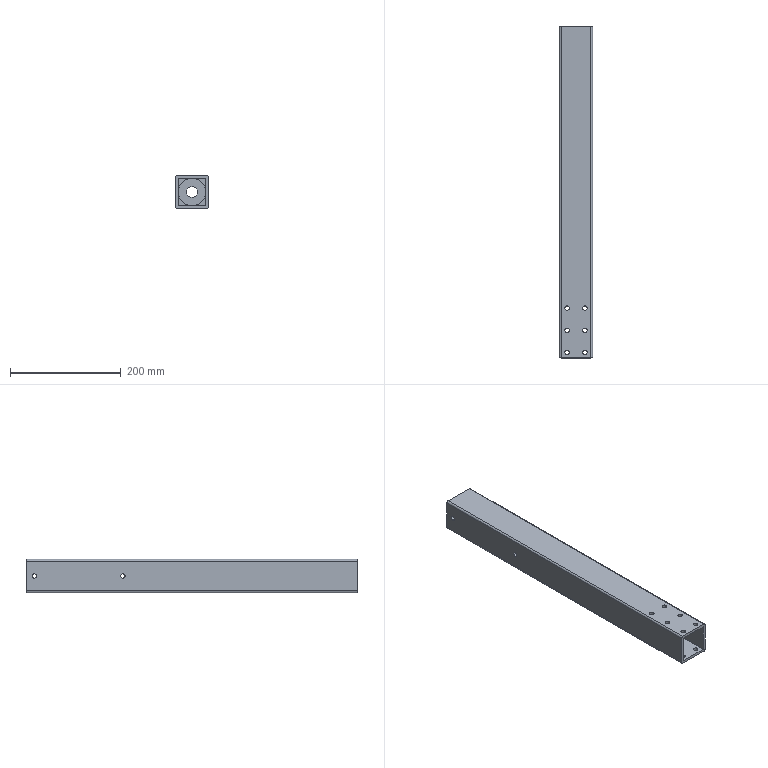Part | SolidWorks | features ICE 9, Fillet 2, Extrusion 1 | 1 solid | 79 faces | box 60 x 600 x 60 mm | volume 948372 mm3 | cylinder 54 | plane 25 | commonest cylinder face diameters 8 x32 5 x8 6 x8 20 x2 40 x2 50 x2